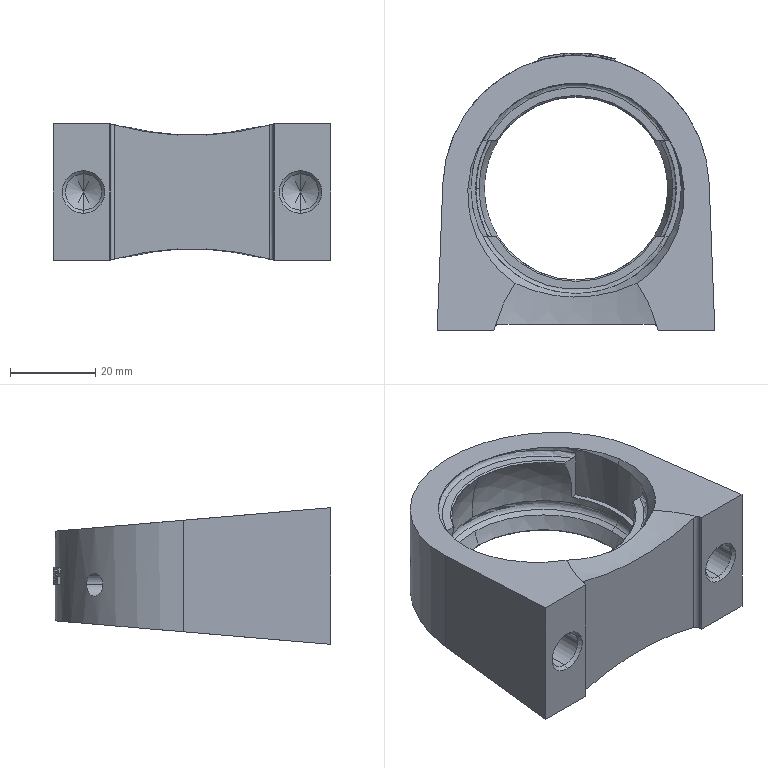Part | SolidWorks | features BaseBody 1 | 1 solid | 192 faces | box 65 x 65 x 32 mm | volume 47548 mm3 | plane 83 | cylinder 70 | cone 23 | torus 12 | sphere 4 | commonest cylinder face diameters 0.129 x14 0.222 x14 0.41 x13 0.126 x10 8.5 x4 49.274 x4